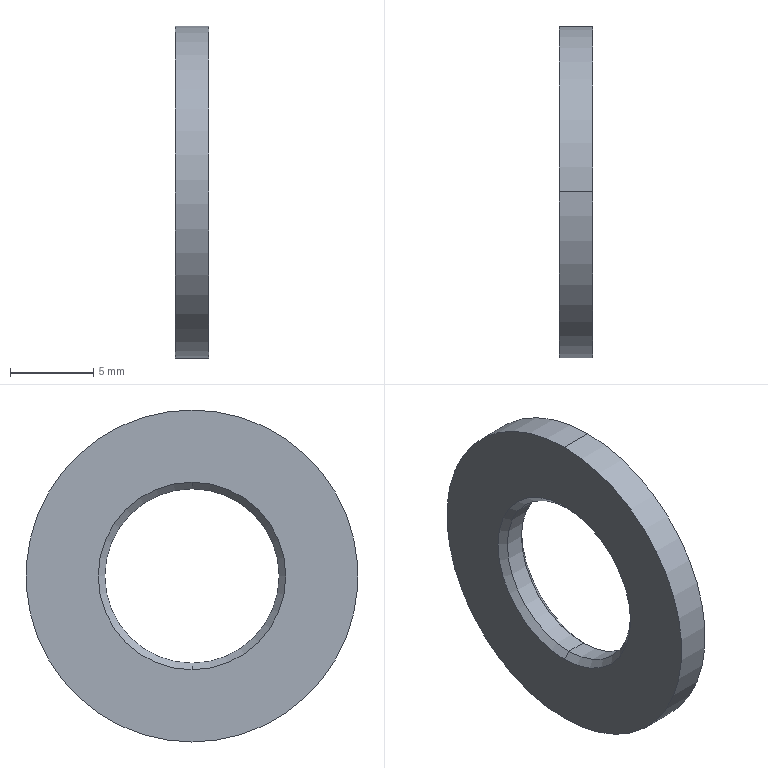Part | STEP file | Microwave Drying Flat Conveyor-plain washer hardened grade a_din_Washer DIN 125 - A 10.5 - 300HV_Default | 1 solid | 10 faces | box 2 x 20 x 20 mm | volume 449.726 mm3 | cylinder 4 | cone 4 | plane 2 | commonest cylinder face diameters 10.5 x2 20 x2
STEP:
#1=CARTESIAN_POINT('',(0.,0.,10.));
#2=VERTEX_POINT('',#1);
#3=CARTESIAN_POINT('',(0.,0.,-10.));
#4=VERTEX_POINT('',#3);
#5=CARTESIAN_POINT('',(0.,0.,0.));
#6=DIRECTION('',(-1.,0.,0.));
#7=DIRECTION('',(0.,0.,1.));
#8=AXIS2_PLACEMENT_3D('',#5,#6,#7);
#9=CIRCLE('',#8,10.);
#10=EDGE_CURVE('',#2,#4,#9,.T.);
#11=ORIENTED_EDGE('',*,*,#10,.T.);
#12=CARTESIAN_POINT('',(-2.,0.,-10.));
#13=VERTEX_POINT('',#12);
#14=CARTESIAN_POINT('',(-34.925,0.,-10.));
#15=DIRECTION('',(-1.,0.,0.));
#16=VECTOR('',#15,1000.);
#17=LINE('',#14,#16);
#18=EDGE_CURVE('',#4,#13,#17,.T.);
#19=ORIENTED_EDGE('',*,*,#18,.T.);
#20=CARTESIAN_POINT('',(-2.,0.,10.));
#21=VERTEX_POINT('',#20);
#22=CARTESIAN_POINT('',(-2.,0.,0.));
#23=DIRECTION('',(1.,0.,0.));
#24=DIRECTION('',(0.,0.,1.));
#25=AXIS2_PLACEMENT_3D('',#22,#23,#24);
#26=CIRCLE('',#25,10.);
#27=EDGE_CURVE('',#13,#21,#26,.T.);
#28=ORIENTED_EDGE('',*,*,#27,.T.);
#29=CARTESIAN_POINT('',(-34.925,0.,10.));
#30=DIRECTION('',(-1.,0.,0.));
#31=VECTOR('',#30,1000.);
#32=LINE('',#29,#31);
#33=EDGE_CURVE('',#2,#21,#32,.T.);
#34=ORIENTED_EDGE('',*,*,#33,.F.);
#35=EDGE_LOOP('',(#11,#19,#28,#34));
#36=FACE_OUTER_BOUND('',#35,.T.);
#37=CARTESIAN_POINT('',(-34.925,0.,0.));
#38=DIRECTION('',(-1.,0.,0.));
#39=DIRECTION('',(0.,0.,1.));
#40=AXIS2_PLACEMENT_3D('',#37,#38,#39);
#41=CYLINDRICAL_SURFACE('',#40,10.);
#42=ADVANCED_FACE('',(#36),#41,.T.);
#43=CARTESIAN_POINT('',(-0.4,0.,5.25));
#44=VERTEX_POINT('',#43);
#45=CARTESIAN_POINT('',(-0.4,0.,-5.25));
#46=VERTEX_POINT('',#45);
#47=CARTESIAN_POINT('',(-0.4,0.,0.));
#48=DIRECTION('',(1.,0.,0.));
#49=DIRECTION('',(0.,0.,-1.));
#50=AXIS2_PLACEMENT_3D('',#47,#48,#49);
#51=CIRCLE('',#50,5.25);
#52=EDGE_CURVE('',#44,#46,#51,.T.);
#53=ORIENTED_EDGE('',*,*,#52,.F.);
#54=CARTESIAN_POINT('',(0.,0.,5.65));
#55=VERTEX_POINT('',#54);
#56=CARTESIAN_POINT('',(0.,0.,5.65));
#57=DIRECTION('',(0.7071,0.,0.7071));
#58=VECTOR('',#57,1000.);
#59=LINE('',#56,#58);
#60=EDGE_CURVE('',#44,#55,#59,.T.);
#61=ORIENTED_EDGE('',*,*,#60,.T.);
#62=CARTESIAN_POINT('',(0.,0.,-5.65));
#63=VERTEX_POINT('',#62);
#64=CARTESIAN_POINT('',(0.,0.,0.));
#65=DIRECTION('',(1.,0.,0.));
#66=DIRECTION('',(0.,0.,-1.));
#67=AXIS2_PLACEMENT_3D('',#64,#65,#66);
#68=CIRCLE('',#67,5.65);
#69=EDGE_CURVE('',#55,#63,#68,.T.);
#70=ORIENTED_EDGE('',*,*,#69,.T.);
#71=CARTESIAN_POINT('',(0.,0.,-5.65));
#72=DIRECTION('',(0.7071,0.,-0.7071));
#73=VECTOR('',#72,1000.);
#74=LINE('',#71,#73);
#75=EDGE_CURVE('',#46,#63,#74,.T.);
#76=ORIENTED_EDGE('',*,*,#75,.F.);
#77=EDGE_LOOP('',(#53,#61,#70,#76));
#78=FACE_OUTER_BOUND('',#77,.T.);
#79=CARTESIAN_POINT('',(0.,0.,0.));
#80=DIRECTION('',(1.,0.,0.));
#81=DIRECTION('',(0.,0.,-1.));
#82=AXIS2_PLACEMENT_3D('',#79,#80,#81);
#83=CONICAL_SURFACE('',#82,5.65,0.7854);
#84=ADVANCED_FACE('',(#78),#83,.F.);
#85=ORIENTED_EDGE('',*,*,#52,.T.);
#86=CARTESIAN_POINT('',(-1.6,0.,-5.25));
#87=VERTEX_POINT('',#86);
#88=CARTESIAN_POINT('',(-34.925,0.,-5.25));
#89=DIRECTION('',(-1.,0.,0.));
#90=VECTOR('',#89,1000.);
#91=LINE('',#88,#90);
#92=EDGE_CURVE('',#46,#87,#91,.T.);
#93=ORIENTED_EDGE('',*,*,#92,.T.);
#94=CARTESIAN_POINT('',(-1.6,0.,5.25));
#95=VERTEX_POINT('',#94);
#96=CARTESIAN_POINT('',(-1.6,0.,0.));
#97=DIRECTION('',(1.,0.,0.));
#98=DIRECTION('',(0.,0.,1.));
#99=AXIS2_PLACEMENT_3D('',#96,#97,#98);
#100=CIRCLE('',#99,5.25);
#101=EDGE_CURVE('',#95,#87,#100,.T.);
#102=ORIENTED_EDGE('',*,*,#101,.F.);
#103=CARTESIAN_POINT('',(-34.925,0.,5.25));
#104=DIRECTION('',(-1.,0.,0.));
#105=VECTOR('',#104,1000.);
#106=LINE('',#103,#105);
#107=EDGE_CURVE('',#44,#95,#106,.T.);
#108=ORIENTED_EDGE('',*,*,#107,.F.);
#109=EDGE_LOOP('',(#85,#93,#102,#108));
#110=FACE_OUTER_BOUND('',#109,.T.);
#111=CARTESIAN_POINT('',(-34.925,0.,0.));
#112=DIRECTION('',(-1.,0.,0.));
#113=DIRECTION('',(0.,0.,1.));
#114=AXIS2_PLACEMENT_3D('',#111,#112,#113);
#115=CYLINDRICAL_SURFACE('',#114,5.25);
#116=ADVANCED_FACE('',(#110),#115,.F.);
#117=ORIENTED_EDGE('',*,*,#101,.T.);
#118=CARTESIAN_POINT('',(-2.,0.,-5.65));
#119=VERTEX_POINT('',#118);
#120=CARTESIAN_POINT('',(-2.,0.,-5.65));
#121=DIRECTION('',(-0.7071,0.,-0.7071));
#122=VECTOR('',#121,1000.);
#123=LINE('',#120,#122);
#124=EDGE_CURVE('',#87,#119,#123,.T.);
#125=ORIENTED_EDGE('',*,*,#124,.T.);
#126=CARTESIAN_POINT('',(-2.,0.,5.65));
#127=VERTEX_POINT('',#126);
#128=CARTESIAN_POINT('',(-2.,0.,0.));
#129=DIRECTION('',(-1.,0.,0.));
#130=DIRECTION('',(0.,0.,1.));
#131=AXIS2_PLACEMENT_3D('',#128,#129,#130);
#132=CIRCLE('',#131,5.65);
#133=EDGE_CURVE('',#119,#127,#132,.T.);
#134=ORIENTED_EDGE('',*,*,#133,.T.);
#135=CARTESIAN_POINT('',(-2.,0.,5.65));
#136=DIRECTION('',(-0.7071,0.,0.7071));
#137=VECTOR('',#136,1000.);
#138=LINE('',#135,#137);
#139=EDGE_CURVE('',#95,#127,#138,.T.);
#140=ORIENTED_EDGE('',*,*,#139,.F.);
#141=EDGE_LOOP('',(#117,#125,#134,#140));
#142=FACE_OUTER_BOUND('',#141,.T.);
#143=CARTESIAN_POINT('',(-2.,0.,0.));
#144=DIRECTION('',(-1.,0.,0.));
#145=DIRECTION('',(0.,0.,1.));
#146=AXIS2_PLACEMENT_3D('',#143,#144,#145);
#147=CONICAL_SURFACE('',#146,5.65,0.7854);
#148=ADVANCED_FACE('',(#142),#147,.F.);
#149=ORIENTED_EDGE('',*,*,#10,.F.);
#150=CARTESIAN_POINT('',(0.,0.,0.));
#151=DIRECTION('',(-1.,0.,0.));
#152=DIRECTION('',(0.,0.,1.));
#153=AXIS2_PLACEMENT_3D('',#150,#151,#152);
#154=CIRCLE('',#153,10.);
#155=EDGE_CURVE('',#4,#2,#154,.T.);
#156=ORIENTED_EDGE('',*,*,#155,.F.);
#157=EDGE_LOOP('',(#149,#156));
#158=FACE_OUTER_BOUND('',#157,.T.);
#159=CARTESIAN_POINT('',(0.,0.,0.));
#160=DIRECTION('',(1.,0.,0.));
#161=DIRECTION('',(0.,0.,-1.));
#162=AXIS2_PLACEMENT_3D('',#159,#160,#161);
#163=CIRCLE('',#162,5.65);
#164=EDGE_CURVE('',#63,#55,#163,.T.);
#165=ORIENTED_EDGE('',*,*,#164,.F.);
#166=ORIENTED_EDGE('',*,*,#69,.F.);
#167=EDGE_LOOP('',(#165,#166));
#168=FACE_BOUND('',#167,.T.);
#169=CARTESIAN_POINT('',(0.,5.25,0.));
#170=DIRECTION('',(-1.,0.,0.));
#171=DIRECTION('',(0.,0.,1.));
#172=AXIS2_PLACEMENT_3D('',#169,#170,#171);
#173=PLANE('',#172);
#174=ADVANCED_FACE('',(#158,#168),#173,.F.);
#175=ORIENTED_EDGE('',*,*,#18,.F.);
#176=ORIENTED_EDGE('',*,*,#155,.T.);
#177=ORIENTED_EDGE('',*,*,#33,.T.);
#178=CARTESIAN_POINT('',(-2.,0.,0.));
#179=DIRECTION('',(1.,0.,0.));
#180=DIRECTION('',(0.,0.,1.));
#181=AXIS2_PLACEMENT_3D('',#178,#179,#180);
#182=CIRCLE('',#181,10.);
#183=EDGE_CURVE('',#21,#13,#182,.T.);
#184=ORIENTED_EDGE('',*,*,#183,.T.);
#185=EDGE_LOOP('',(#175,#176,#177,#184));
#186=FACE_OUTER_BOUND('',#185,.T.);
#187=CARTESIAN_POINT('',(-34.925,0.,0.));
#188=DIRECTION('',(-1.,0.,0.));
#189=DIRECTION('',(0.,0.,1.));
#190=AXIS2_PLACEMENT_3D('',#187,#188,#189);
#191=CYLINDRICAL_SURFACE('',#190,10.);
#192=ADVANCED_FACE('',(#186),#191,.T.);
#193=ORIENTED_EDGE('',*,*,#60,.F.);
#194=CARTESIAN_POINT('',(-0.4,0.,0.));
#195=DIRECTION('',(1.,0.,0.));
#196=DIRECTION('',(0.,0.,-1.));
#197=AXIS2_PLACEMENT_3D('',#194,#195,#196);
#198=CIRCLE('',#197,5.25);
#199=EDGE_CURVE('',#46,#44,#198,.T.);
#200=ORIENTED_EDGE('',*,*,#199,.F.);
#201=ORIENTED_EDGE('',*,*,#75,.T.);
#202=ORIENTED_EDGE('',*,*,#164,.T.);
#203=EDGE_LOOP('',(#193,#200,#201,#202));
#204=FACE_OUTER_BOUND('',#203,.T.);
#205=CARTESIAN_POINT('',(0.,0.,0.));
#206=DIRECTION('',(1.,0.,0.));
#207=DIRECTION('',(0.,0.,-1.));
#208=AXIS2_PLACEMENT_3D('',#205,#206,#207);
#209=CONICAL_SURFACE('',#208,5.65,0.7854);
#210=ADVANCED_FACE('',(#204),#209,.F.);
#211=ORIENTED_EDGE('',*,*,#183,.F.);
#212=ORIENTED_EDGE('',*,*,#27,.F.);
#213=EDGE_LOOP('',(#211,#212));
#214=FACE_OUTER_BOUND('',#213,.T.);
#215=CARTESIAN_POINT('',(-2.,0.,0.));
#216=DIRECTION('',(-1.,0.,0.));
#217=DIRECTION('',(0.,0.,1.));
#218=AXIS2_PLACEMENT_3D('',#215,#216,#217);
#219=CIRCLE('',#218,5.65);
#220=EDGE_CURVE('',#127,#119,#219,.T.);
#221=ORIENTED_EDGE('',*,*,#220,.F.);
#222=ORIENTED_EDGE('',*,*,#133,.F.);
#223=EDGE_LOOP('',(#221,#222));
#224=FACE_BOUND('',#223,.T.);
#225=CARTESIAN_POINT('',(-2.,10.,0.));
#226=DIRECTION('',(1.,0.,0.));
#227=DIRECTION('',(0.,0.,-1.));
#228=AXIS2_PLACEMENT_3D('',#225,#226,#227);
#229=PLANE('',#228);
#230=ADVANCED_FACE('',(#214,#224),#229,.F.);
#231=ORIENTED_EDGE('',*,*,#92,.F.);
#232=ORIENTED_EDGE('',*,*,#199,.T.);
#233=ORIENTED_EDGE('',*,*,#107,.T.);
#234=CARTESIAN_POINT('',(-1.6,0.,0.));
#235=DIRECTION('',(1.,0.,0.));
#236=DIRECTION('',(0.,0.,1.));
#237=AXIS2_PLACEMENT_3D('',#234,#235,#236);
#238=CIRCLE('',#237,5.25);
#239=EDGE_CURVE('',#87,#95,#238,.T.);
#240=ORIENTED_EDGE('',*,*,#239,.F.);
#241=EDGE_LOOP('',(#231,#232,#233,#240));
#242=FACE_OUTER_BOUND('',#241,.T.);
#243=CARTESIAN_POINT('',(-34.925,0.,0.));
#244=DIRECTION('',(-1.,0.,0.));
#245=DIRECTION('',(0.,0.,1.));
#246=AXIS2_PLACEMENT_3D('',#243,#244,#245);
#247=CYLINDRICAL_SURFACE('',#246,5.25);
#248=ADVANCED_FACE('',(#242),#247,.F.);
#249=ORIENTED_EDGE('',*,*,#124,.F.);
#250=ORIENTED_EDGE('',*,*,#239,.T.);
#251=ORIENTED_EDGE('',*,*,#139,.T.);
#252=ORIENTED_EDGE('',*,*,#220,.T.);
#253=EDGE_LOOP('',(#249,#250,#251,#252));
#254=FACE_OUTER_BOUND('',#253,.T.);
#255=CARTESIAN_POINT('',(-2.,0.,0.));
#256=DIRECTION('',(-1.,0.,0.));
#257=DIRECTION('',(0.,0.,1.));
#258=AXIS2_PLACEMENT_3D('',#255,#256,#257);
#259=CONICAL_SURFACE('',#258,5.65,0.7854);
#260=ADVANCED_FACE('',(#254),#259,.F.);
#261=CLOSED_SHELL('',(#42,#84,#116,#148,#174,#192,#210,#230,#248,#260));
#262=MANIFOLD_SOLID_BREP('',#261);
#263=CARTESIAN_POINT('',(0.,0.,0.));
#264=DIRECTION('',(0.,0.,1.));
#265=DIRECTION('',(1.,0.,0.));
#266=AXIS2_PLACEMENT_3D('',#263,#264,#265);
#267=(LENGTH_UNIT()NAMED_UNIT(*)SI_UNIT(.MILLI.,.METRE.));
#268=UNCERTAINTY_MEASURE_WITH_UNIT(LENGTH_MEASURE(0.00001),#267,'','');
#269=(NAMED_UNIT(*)PLANE_ANGLE_UNIT()SI_UNIT($,.RADIAN.));
#270=(NAMED_UNIT(*)SI_UNIT($,.STERADIAN.)SOLID_ANGLE_UNIT());
#271=(GEOMETRIC_REPRESENTATION_CONTEXT(3)GLOBAL_UNCERTAINTY_ASSIGNED_CONTEXT((#268))GLOBAL_UNIT_ASSIGNED_CONTEXT((#267,#269,#270))REPRESENTATION_CONTEXT('',''));
#272=ADVANCED_BREP_SHAPE_REPRESENTATION('',(#262,#266),#271);